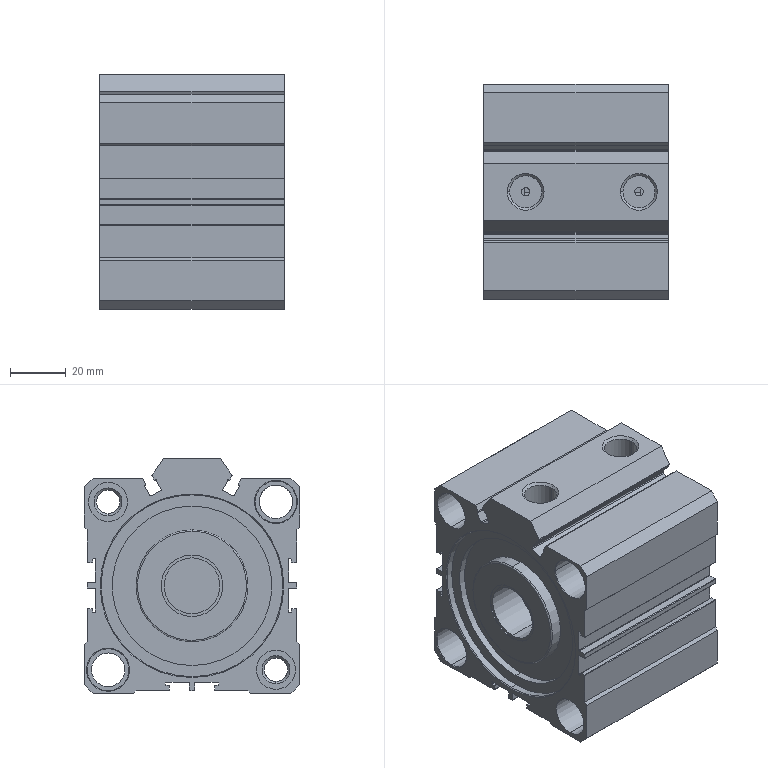Part | SolidWorks | features BaseBody 1 | 1 solid | 244 faces | box 66 x 77 x 84 mm | volume 195139 mm3 | cylinder 113 | plane 99 | cone 30 | spline 2 | commonest cylinder face diameters 0.4 x41 0.8 x8 8.376 x8 14 x8 0.2 x4 3 x4